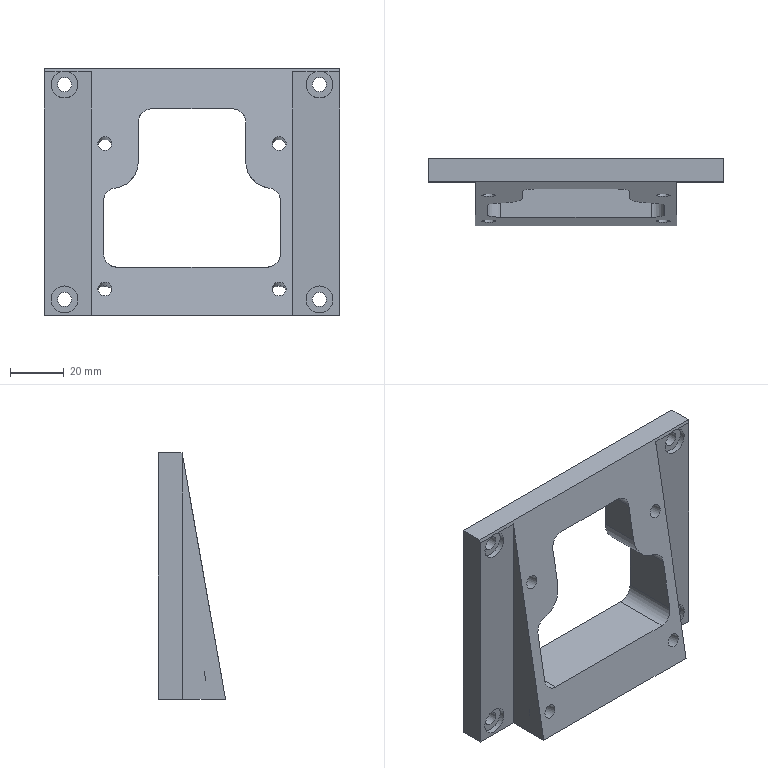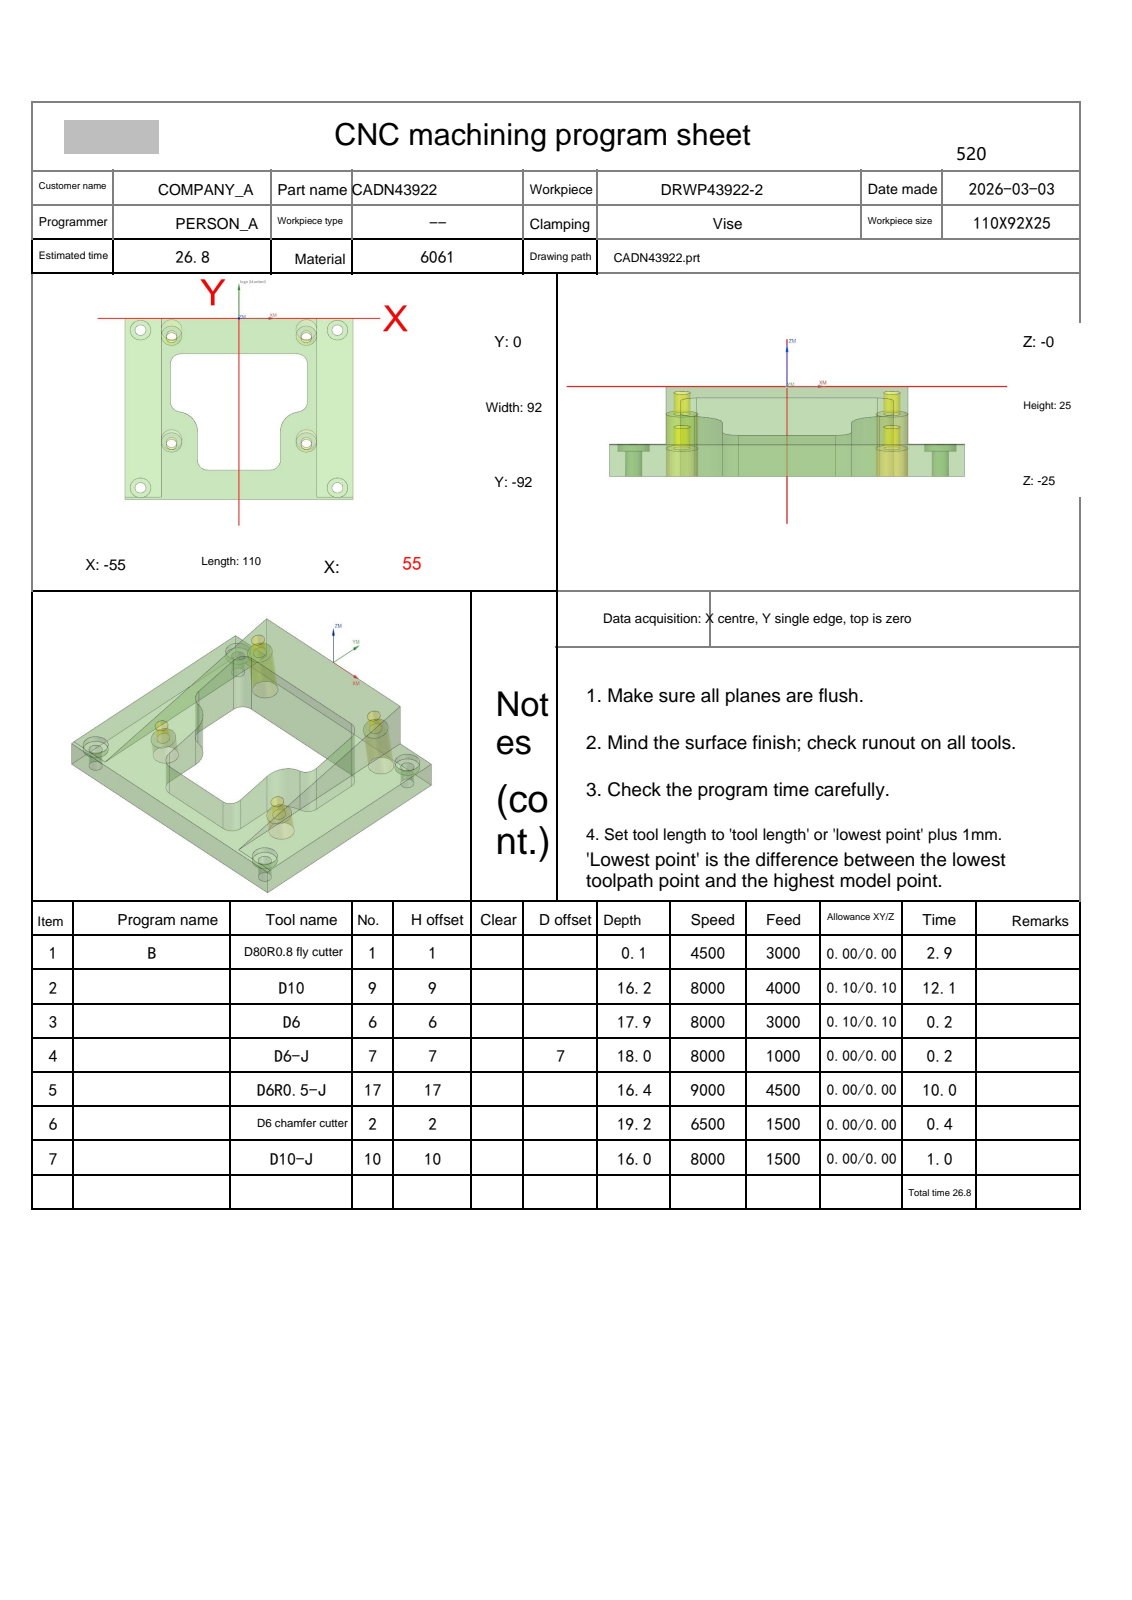NC program | NX | posted by the shop | part box 110 x 25 x 92 mm
Lines 5947 to 7507 of 14355:
N5 T17 M06
(D6R0.5-J  D=6. R=0.5 H=17 ce=0.00 di=0.00)
G00 G90 G54 X38.576 Y-2.64 M03 S9000
G43 H17 Z14.5
M08
Z1.2
G01 Z-.017 F4500.
X37.5 Y-2.642
X-37.5
X-38.576 Y-2.64
Y-2.691 Z-.026
Y-2.739 Z-.035
X-37.5 Y-2.741
X37.5
X38.576 Y-2.739
X38.577 Y-2.79 Z-.043
Y-2.837 Z-.052
X37.5 Y-2.839
X-37.5
X-38.577 Y-2.837
Y-2.888 Z-.061
Y-2.936 Z-.069
X-37.5 Y-2.938
X37.5
X38.577 Y-2.936
X38.578 Y-2.987 Z-.078
Y-3.034 Z-.087
X37.5 Y-3.036
X-37.5
X-38.578 Y-3.034
Y-3.085 Z-.096
X-38.579 Y-3.133 Z-.104
X-37.5 Y-3.135
X37.5
X38.579 Y-3.133
Y-3.184 Z-.113
Y-3.231 Z-.122
X37.5 Y-3.233
X-37.5
X-38.579 Y-3.231
Y-3.282 Z-.13
X-38.58 Y-3.33 Z-.139
X-37.5 Y-3.332
X37.5
X38.58 Y-3.33
Y-3.381 Z-.148
Y-3.428 Z-.156
X37.5 Y-3.43
X-37.5
X-38.58 Y-3.428
Y-3.479 Z-.165
X-38.581 Y-3.527 Z-.174
X-37.5 Y-3.529
X37.5
X38.581 Y-3.527
Y-3.578 Z-.182
Y-3.625 Z-.191
X37.5 Y-3.627
X-37.5
X-38.581 Y-3.625
Y-3.676 Z-.2
X-38.582 Y-3.723 Z-.208
X-37.5 Y-3.726
X37.5
X38.582 Y-3.723
Y-3.775 Z-.217
Y-3.822 Z-.226
X37.5 Y-3.824
X-37.5
X-38.582 Y-3.822
X-38.583 Y-3.873 Z-.234
Y-3.92 Z-.243
X-37.5 Y-3.922
X37.5
X38.583 Y-3.92
Y-3.972 Z-.252
Y-4.019 Z-.26
X37.5 Y-4.021
X-37.5
X-38.583 Y-4.019
X-38.584 Y-4.07 Z-.269
Y-4.117 Z-.278
X-37.5 Y-4.119
X37.5
X38.584 Y-4.117
Y-4.169 Z-.287
Y-4.216 Z-.295
X37.5 Y-4.218
X-37.5
X-38.584 Y-4.216
X-38.585 Y-4.267 Z-.304
Y-4.314 Z-.313
X-37.5 Y-4.316
X37.5
X38.585 Y-4.314
Y-4.366 Z-.321
Y-4.413 Z-.33
X37.5 Y-4.415
X-37.5
X-38.585 Y-4.413
X-38.586 Y-4.464 Z-.339
Y-4.511 Z-.347
X-37.5 Y-4.513
X37.5
X38.586 Y-4.511
Y-4.563 Z-.356
Y-4.61 Z-.365
X37.5 Y-4.612
X-37.5
X-38.586 Y-4.61
Y-4.661 Z-.373
X-38.587 Y-4.708 Z-.382
X-37.5 Y-4.71
X37.5
X38.587 Y-4.708
Y-4.76 Z-.391
Y-4.807 Z-.399
X37.5 Y-4.809
X-37.5
X-38.587 Y-4.807
Y-4.858 Z-.408
X-38.588 Y-4.905 Z-.417
X-37.5 Y-4.907
X37.5
X38.588 Y-4.905
Y-4.957 Z-.425
Y-5.004 Z-.434
X37.5 Y-5.006
X-37.5
X-38.588 Y-5.004
Y-5.055 Z-.443
Y-5.102 Z-.451
X-37.5 Y-5.104
X37.5
X38.588 Y-5.102
X38.589 Y-5.153 Z-.46
Y-5.201 Z-.469
X37.5 Y-5.203
X-37.5
X-38.589 Y-5.201
Y-5.252 Z-.478
Y-5.299 Z-.486
X-37.5 Y-5.301
X37.5
X38.589 Y-5.299
Y-5.35 Z-.495
Y-5.398 Z-.504
X37.5 Y-5.4
X-37.5
X-38.589 Y-5.398
X-38.59 Y-5.449 Z-.512
Y-5.496 Z-.521
X-37.5 Y-5.498
X37.5
X38.59 Y-5.496
Y-5.547 Z-.53
Y-5.595 Z-.538
X37.5 Y-5.597
X-37.5
X-38.59 Y-5.595
Y-5.646 Z-.547
X-38.591 Y-5.693 Z-.556
X-37.5 Y-5.695
X37.5
X38.591 Y-5.693
Y-5.744 Z-.564
Y-5.792 Z-.573
X37.5 Y-5.794
X-37.5
X-38.591 Y-5.792
Y-5.843 Z-.582
Y-5.89 Z-.59
X-37.5 Y-5.892
X37.5
X38.591 Y-5.89
X38.592 Y-5.941 Z-.599
Y-5.989 Z-.608
X37.5 Y-5.991
X-37.5
X-38.592 Y-5.989
Y-6.04 Z-.616
Y-6.087 Z-.625
X-37.5 Y-6.089
X37.5
X38.592 Y-6.087
Y-6.138 Z-.634
X38.593 Y-6.186 Z-.642
X37.5 Y-6.188
X-37.5
X-38.593 Y-6.186
Y-6.237 Z-.651
Y-6.284 Z-.66
X-37.5 Y-6.286
X37.5
X38.593 Y-6.284
Y-6.335 Z-.669
Y-6.383 Z-.677
X37.5 Y-6.384
X-37.5
X-38.593 Y-6.383
Y-6.434 Z-.686
X-38.594 Y-6.481 Z-.695
X-37.5 Y-6.483
X37.5
X38.594 Y-6.481
Y-6.532 Z-.703
Y-6.58 Z-.712
X37.5 Y-6.581
X-37.5
X-38.594 Y-6.58
Y-6.631 Z-.721
Y-6.678 Z-.729
X-37.5 Y-6.68
X37.5
X38.594 Y-6.678
Y-6.729 Z-.738
Y-6.777 Z-.747
X37.5 Y-6.778
X-37.5
X-38.594 Y-6.777
Y-6.828 Z-.755
Y-6.875 Z-.764
X-37.5 Y-6.877
X37.5
X38.594 Y-6.875
X38.595 Y-6.926 Z-.773
Y-6.974 Z-.781
X37.5 Y-6.975
X-37.5
X-38.595 Y-6.974
Y-7.025 Z-.79
Y-7.072 Z-.799
X-37.5 Y-7.074
X37.5
X38.595 Y-7.072
Y-7.123 Z-.807
Y-7.171 Z-.816
X37.5 Y-7.172
X-37.5
X-38.595 Y-7.171
Y-7.222 Z-.825
Y-7.269 Z-.834
X-37.5 Y-7.271
X37.5
X38.595 Y-7.269
Y-7.32 Z-.842
Y-7.368 Z-.851
X37.5 Y-7.369
X-37.5
X-38.595 Y-7.368
X-38.596 Y-7.419 Z-.86
Y-7.466 Z-.868
X-37.5 Y-7.468
X37.5
X38.596 Y-7.466
Y-7.517 Z-.877
Y-7.565 Z-.886
X37.5 Y-7.566
X-37.5
X-38.596 Y-7.565
Y-7.616 Z-.894
Y-7.663 Z-.903
X-37.5 Y-7.665
X37.5
X38.596 Y-7.663
Y-7.714 Z-.912
Y-7.762 Z-.92
X37.5 Y-7.763
X-37.5
X-38.596 Y-7.762
Y-7.812 Z-.929
Y-7.86 Z-.938
X-37.5 Y-7.862
X37.5
X38.596 Y-7.86
X38.597 Y-7.911 Z-.946
Y-7.958 Z-.955
X37.5 Y-7.96
X-37.5
X-38.597 Y-7.958
Y-8.009 Z-.964
Y-8.057 Z-.972
X-37.5 Y-8.059
X37.5
X38.597 Y-8.057
Y-8.108 Z-.981
Y-8.155 Z-.99
X37.5 Y-8.157
X-37.5
X-38.597 Y-8.155
Y-8.206 Z-.998
Y-8.254 Z-1.007
X-37.5 Y-8.256
X37.5
X38.597 Y-8.254
Y-8.305 Z-1.016
X38.598 Y-8.352 Z-1.025
X37.5 Y-8.354
X-37.5
X-38.597 Y-8.352
Y-8.403 Z-1.033
Y-8.451 Z-1.042
X-37.5 Y-8.453
X37.5
X38.598 Y-8.451
Y-8.502 Z-1.051
Y-8.549 Z-1.059
X37.5 Y-8.551
X-37.5
X-38.598 Y-8.549
Y-8.6 Z-1.068
Y-8.648 Z-1.077
X-37.5 Y-8.65
X37.5
X38.598 Y-8.648
Y-8.699 Z-1.085
Y-8.746 Z-1.094
X37.5 Y-8.748
X-37.5
X-38.598 Y-8.746
Y-8.797 Z-1.103
Y-8.845 Z-1.111
X-37.5 Y-8.847
X37.5
X38.598 Y-8.845
Y-8.896 Z-1.12
Y-8.943 Z-1.129
X37.5 Y-8.945
X-37.5
X-38.598 Y-8.943
Y-8.994 Z-1.137
Y-9.042 Z-1.146
X-37.5 Y-9.043
X37.5
X38.598 Y-9.042
Y-9.093 Z-1.155
Y-9.14 Z-1.163
X37.5 Y-9.142
X-37.5
X-38.598 Y-9.14
Y-9.191 Z-1.172
Y-9.239 Z-1.181
X-37.5 Y-9.24
X37.5
X38.598 Y-9.239
Y-9.29 Z-1.189
Y-9.337 Z-1.198
X37.5 Y-9.339
X-37.5
X-38.598 Y-9.337
Y-9.388 Z-1.207
Y-9.436 Z-1.216
X-37.5 Y-9.437
X37.5
X38.598 Y-9.436
Y-9.487 Z-1.224
Y-9.534 Z-1.233
X37.5 Y-9.536
X-37.5
X-38.599 Y-9.534
Y-9.585 Z-1.242
Y-9.633 Z-1.25
X-37.5 Y-9.634
X37.5
X38.599 Y-9.633
Y-9.684 Z-1.259
Y-9.731 Z-1.268
X37.5 Y-9.733
X-37.5
X-38.599 Y-9.731
Y-9.782 Z-1.276
Y-9.83 Z-1.285
X-37.5 Y-9.831
X37.5
X38.599 Y-9.83
Y-9.881 Z-1.294
Y-9.928 Z-1.302
X37.5 Y-9.93
X-37.5
X-38.599 Y-9.928
Y-9.979 Z-1.311
Y-10.027 Z-1.32
X-37.5 Y-10.028
X37.5
X38.599 Y-10.027
Y-10.078 Z-1.328
Y-10.125 Z-1.337
X37.5 Y-10.127
X-37.5
X-38.599 Y-10.125
Y-10.176 Z-1.346
Y-10.224 Z-1.354
X-37.5 Y-10.225
X37.5
X38.599 Y-10.224
Y-10.274 Z-1.363
Y-10.322 Z-1.372
X37.5 Y-10.324
X-37.5
X-38.599 Y-10.322
Y-10.373 Z-1.381
Y-10.421 Z-1.389
X-37.5 Y-10.422
X37.5
X38.599 Y-10.421
Y-10.471 Z-1.398
Y-10.519 Z-1.407
X37.5 Y-10.521
X-37.5
X-38.599 Y-10.519
Y-10.57 Z-1.415
Y-10.618 Z-1.424
X-37.5 Y-10.619
X37.5
X38.599 Y-10.618
Y-10.668 Z-1.433
Y-10.716 Z-1.441
X37.5 Y-10.718
X-37.5
X-38.599 Y-10.716
Y-10.767 Z-1.45
Y-10.814 Z-1.459
X-37.5 Y-10.816
X37.5
X38.599 Y-10.814
Y-10.865 Z-1.467
Y-10.913 Z-1.476
X37.5 Y-10.915
X-37.5
X-38.599 Y-10.913
Y-10.964 Z-1.485
Y-11.011 Z-1.493
X-37.5 Y-11.013
X37.5
X38.599 Y-11.011
Y-11.062 Z-1.502
Y-11.11 Z-1.511
X37.5 Y-11.112
X34.721
X32.994 Y-11.109
G03 X32.501 Y-11.091 I-.493 J-6.934
X32.006 Y-11.109 I0.0 J-6.951
G01 X30.279 Y-11.112
X-30.279
X-32.006 Y-11.109
G03 X-32.501 Y-11.091 I-.495 J-6.928
X-32.994 Y-11.109 I0.0 J-6.946
G01 X-34.721 Y-11.112
X-37.5
X-38.599 Y-11.11
Y-11.161 Z-1.519
Y-11.208 Z-1.528
X-37.5 Y-11.21
X-34.778
X-33.203 Y-11.209
G02 X-32.499 Y-11.159 I.704 J-4.954
X-31.789 Y-11.209 I0.0 J-5.004
G01 X-30.222 Y-11.21
X30.222
X31.789 Y-11.209
G02 X32.499 Y-11.159 I.71 J-4.956
X33.204 Y-11.209 I0.0 J-5.006
G01 X34.778 Y-11.21
X37.5
X38.599 Y-11.208
Y-11.259 Z-1.537
Y-11.307 Z-1.545
X37.5 Y-11.309
X34.825
X33.335 Y-11.303
G03 X32.499 Y-11.223 I-.836 J-4.329
X31.66 Y-11.303 I0.0 J-4.409
G01 X30.175 Y-11.309
X-30.175
X-31.66 Y-11.303
G03 X-32.499 Y-11.223 I-.839 J-4.328
X-33.335 Y-11.303 I0.0 J-4.409
G01 X-34.825 Y-11.309
X-37.5
X-38.599 Y-11.307
Y-11.358 Z-1.554
Y-11.405 Z-1.563
X-37.5 Y-11.407
X-34.871
X-33.467 Y-11.404
X-32.49 Y-11.253
X-31.532 Y-11.403
X-30.129 Y-11.407
X30.129
X31.532 Y-11.403
X32.49 Y-11.253
X33.467 Y-11.404
X34.871 Y-11.407
X37.5
X38.6 Y-11.405
Y-11.456 Z-1.572
Y-11.504 Z-1.58
X37.5 Y-11.506
X34.918
X33.565 Y-11.504
G02 X32.49 Y-11.308 I.169 J3.981
X31.43 Y-11.505 I-1.183 J3.427
G01 X30.082 Y-11.506
X-30.082
X-31.43 Y-11.505
G02 X-32.49 Y-11.308 I.122 J3.616
X-33.565 Y-11.504 I-1.244 J3.785
G01 X-34.918 Y-11.506
X-37.5
X-38.599 Y-11.504
Y-11.555 Z-1.589
Y-11.602 Z-1.598
X-37.5 Y-11.604
X-34.955
X-33.637 Y-11.6
G03 X-32.49 Y-11.363 I-.32 J4.442
X-31.36 Y-11.601 I1.353 J3.628
G01 X-30.045 Y-11.604
X30.045
X31.36 Y-11.601
G03 X32.49 Y-11.363 I-.223 J3.865
X33.637 Y-11.6 I1.465 J4.199
G01 X34.955 Y-11.604
X37.5
X38.6 Y-11.602
Y-11.653 Z-1.606
Y-11.701 Z-1.615
X37.5 Y-11.702
X34.982
X33.709 Y-11.698
X33.661 Y-11.699
G02 X32.597 Y-11.445 I0.0 J2.36
G01 X32.5 Y-11.418
X32.404 Y-11.445
G02 X31.335 Y-11.699 I-1.069 J2.123
G01 X31.29
X30.018 Y-11.702
X-30.018
X-31.29 Y-11.699
X-31.335
G02 X-32.404 Y-11.445 I0.0 J2.377
G01 X-32.501 Y-11.418
X-32.598 Y-11.445
G02 X-33.66 Y-11.699 I-1.063 J2.102
G01 X-33.709 Y-11.698
X-34.982 Y-11.702
X-37.5
X-38.6 Y-11.701
Y-11.752 Z-1.624
Y-11.799 Z-1.632
X-37.5 Y-11.801
X-35.009
X-33.778 Y-11.798
X-33.757
G03 X-32.5 Y-11.478 I0.0 J2.631
X-31.245 Y-11.798 I1.255 J2.303
G01 X-31.223
X-29.991 Y-11.801
X29.991
X31.223 Y-11.798
X31.24
G03 X32.502 Y-11.479 I0.0 J2.66
X33.756 Y-11.798 I1.254 J2.309
G01 X33.778
X35.009 Y-11.801
X37.5
X38.6 Y-11.799
Y-11.85 Z-1.641
Y-11.898 Z-1.65
X37.5 Y-11.899
X35.036
X33.817 Y-11.897
G02 X32.502 Y-11.555 I.026 J2.8
X31.186 Y-11.896 I-1.353 J2.51
G01 X29.964 Y-11.899
X-29.964
X-31.186 Y-11.896
G02 X-32.5 Y-11.554 I.032 J2.815
X-33.817 Y-11.897 I-1.343 J2.458
G01 X-35.036 Y-11.899
X-37.5
X-38.6 Y-11.898
Y-11.949 Z-1.658
Y-11.996 Z-1.667
X-37.5 Y-11.998
X-35.062
X-33.857 Y-11.997
G03 X-32.5 Y-11.629 I-.028 J2.793
X-31.149 Y-11.996 I1.382 J2.421
G01 X-29.939 Y-11.998
X29.939
X31.149 Y-11.996
G03 X32.502 Y-11.63 I-.025 J2.781
X33.857 Y-11.997 I1.376 J2.398
G01 X35.062 Y-11.998
X37.5
X38.6 Y-11.996
Y-12.047 Z-1.676
Y-12.095 Z-1.684
X37.5 Y-12.096
X35.075
X33.889
G02 X32.502 Y-11.706 I.168 J3.259
X31.112 Y-12.096 I-1.607 J3.056
G01 X29.925
X-29.925
X-31.112
G02 X-32.5 Y-11.705 I.18 J3.296
X-33.889 Y-12.096 I-1.56 J2.877
G01 X-35.075
X-37.5
X-38.6 Y-12.095
Y-12.146 Z-1.693
Y-12.193 Z-1.702
X-37.5 Y-12.195
X-35.088
X-33.907
G03 X-32.5 Y-11.781 I-.001 J2.601
X-31.093 Y-12.195 I1.409 J2.191
G01 X-29.912
X29.912
X31.093
G03 X32.502 Y-11.782 I-.008 J2.637
X33.907 Y-12.195 I1.405 J2.186
G01 X35.088
X37.5
X38.6 Y-12.193
Y-12.244 Z-1.71
Y-12.292 Z-1.719
X37.5 Y-12.293
X35.094
X33.92
G02 X32.502 Y-11.873 I.044 J2.754
X31.08 Y-12.293 I-1.477 J2.383
G01 X29.906
X-29.906
X-31.08
G02 X-32.5 Y-11.872 I.048 J2.766
X-33.92 Y-12.293 I-1.464 J2.333
G01 X-35.094
X-37.5
X-38.6 Y-12.292
Y-12.343 Z-1.728
Y-12.39 Z-1.736
X-37.5 Y-12.392
X-35.098
X-33.933 Y-12.391
G03 X-32.5 Y-11.965 I-.014 J2.67
X-31.067 Y-12.391 I1.447 J2.243
G01 X-29.902 Y-12.392
X29.902
X31.067 Y-12.391
G03 X32.502 Y-11.967 I-.02 J2.701
X33.933 Y-12.391 I1.458 J2.291
G01 X35.098 Y-12.392
X37.5
X38.6 Y-12.39
Y-12.441 Z-1.745
Y-12.489 Z-1.754
X37.5 Y-12.49
X35.098
X33.943
X33.904
G02 X32.579 Y-12.094 I0.0 J2.412
G01 X32.529 Y-12.063
X32.47
X32.42 Y-12.094
G02 X31.096 Y-12.49 I-1.324 J2.014
G01 X31.057
X29.902
X-29.902
X-31.057
X-31.095
G02 X-32.43 Y-12.087 I0.0 J2.411
G01 X-32.473 Y-12.059
X-32.526
X-32.569 Y-12.087
G02 X-33.903 Y-12.49 I-1.334 J2.009
G01 X-33.942
X-35.098
X-37.5
X-38.6 Y-12.489
Y-12.54 Z-1.763
Y-12.587 Z-1.771
X-37.5 Y-12.589
X-35.093
X-33.922 Y-12.588
X-33.914
G03 X-32.5 Y-12.156 I0.0 J2.531
X-31.084 Y-12.589 I1.416 J2.103
G01 X-31.076
X-29.907
X29.907
X31.076
X31.079
G03 X32.502 Y-12.157 I0.0 J2.565
X33.914 Y-12.588 I1.412 J2.098
G01 X33.923
X35.093 Y-12.589
X37.5
X38.6 Y-12.587
Y-12.638 Z-1.78
Y-12.686 Z-1.789
X37.5 Y-12.687
X35.086
X33.903
G02 X32.502 Y-12.272 I.003 J2.581
X31.094 Y-12.687 I-1.416 J2.203
G01 X29.914
X-29.914
X-31.094
G02 X-32.5 Y-12.27 I.002 J2.588
X-33.903 Y-12.687 I-1.406 J2.166
G01 X-35.086
X-37.5
X-38.6 Y-12.686
Y-12.737 Z-1.797
Y-12.784 Z-1.806
X-37.5 Y-12.786
X-35.073
X-33.883
X-33.881
G03 X-32.5 Y-12.384 I0.0 J2.579
X-31.121 Y-12.785 I1.379 J2.171
G01 X-31.114
X-29.927 Y-12.786
X29.927
X31.114 Y-12.785
X31.116
G03 X32.502 Y-12.386 I0.0 J2.602
X33.881 Y-12.786 I1.379 J2.177
G01 X33.883
X35.073
X37.5
X38.6 Y-12.784
Y-12.835 Z-1.815
Y-12.883 Z-1.823
X37.5 Y-12.884
X35.059
X33.85 Y-12.883
X33.841
G02 X32.502 Y-12.501 I0.0 J2.54
X31.152 Y-12.882 I-1.35 J2.205
G01 X29.941 Y-12.884
X-29.941
X-31.151 Y-12.882
X-31.165
G02 X-32.5 Y-12.5 I0.0 J2.525
X-33.85 Y-12.883 I-1.353 J2.201
G01 X-35.059 Y-12.884
X-37.5
X-38.6 Y-12.883
Y-12.933 Z-1.832
Y-12.981 Z-1.841
X-37.5 Y-12.983
X-35.032
X-33.806 Y-12.98
X-33.799
G03 X-32.5 Y-12.625 I0.0 J2.553
X-31.204 Y-12.979 I1.296 J2.19
G01 X-31.194
X-29.968 Y-12.983
X29.968
X31.194 Y-12.979
X31.199
G03 X32.502 Y-12.626 I0.0 J2.578
X33.798 Y-12.98 I1.296 J2.197
G01 X33.806
X35.032 Y-12.983
X37.5
X38.6 Y-12.981
Y-13.032 Z-1.849
Y-13.08 Z-1.858
X37.5 Y-13.081
X35.006
X33.762 Y-13.078
X33.739
G02 X32.502 Y-12.75 I0.0 J2.498
X31.257 Y-13.078 I-1.245 J2.202
G01 X31.238 Y-13.077
X29.994 Y-13.081
X-29.994
X-31.238 Y-13.077
X-31.262 Y-13.078
G02 X-32.5 Y-12.749 I0.0 J2.497
X-33.739 Y-13.078 I-1.239 J2.172
G01 X-33.762
X-35.006 Y-13.081
X-37.5
X-38.6 Y-13.08
Y-13.13 Z-1.867
Y-13.178 Z-1.875
X-37.5 Y-13.18
X-34.979
X-33.716 Y-13.177
X-33.707
G03 X-32.49 Y-12.883 I0.0 J2.668
X-31.316 Y-13.177 I1.174 J2.196
G01 X-31.284
X-30.021 Y-13.18
X30.021
X31.284 Y-13.177
X31.316
G03 X32.49 Y-12.883 I0.0 J2.49
G01 X33.527 Y-13.173
X33.716 Y-13.177
X34.979 Y-13.18
X37.5
X38.6 Y-13.178
Y-13.229 Z-1.884
Y-13.277 Z-1.893
X37.5 Y-13.278
X34.952
X33.637 Y-13.275
X33.527 Y-13.274
X32.49 Y-13.019
X31.453 Y-13.275
X31.361 Y-13.276
X30.048 Y-13.278
X-30.048
X-31.361 Y-13.276
X-31.453 Y-13.275
X-32.49 Y-13.019
X-33.527 Y-13.274
X-33.637 Y-13.275
X-34.952 Y-13.278
X-37.5
X-38.6 Y-13.277
Y-13.327 Z-1.901
Y-13.375 Z-1.91
X-37.5 Y-13.377
X-34.912
X-33.558 Y-13.376
X-32.49 Y-13.156
X-31.438 Y-13.376
X-30.088 Y-13.377
X30.088
X31.438 Y-13.376
X32.49 Y-13.156
X33.558 Y-13.376
X34.912 Y-13.377
X37.5
X38.6 Y-13.375
Y-13.426 Z-1.919
Y-13.473 Z-1.927
X37.5 Y-13.475
X34.865
X33.467 Y-13.472
G03 X32.499 Y-13.362 I-.968 J-4.208
X31.533 Y-13.472 I0.0 J-4.318
G01 X30.135 Y-13.475
X-30.135
X-31.533 Y-13.472
G03 X-32.499 Y-13.362 I-.966 J-4.208
X-33.467 Y-13.472 I0.0 J-4.318
G01 X-34.865 Y-13.475
X-37.5
X-38.6 Y-13.473
Y-13.524 Z-1.936
Y-13.572 Z-1.945
X-37.5 Y-13.574
X-34.819
X-33.338 Y-13.57
G02 X-32.5 Y-13.49 I.838 J-4.356
X-31.66 Y-13.57 I0.0 J-4.436
G01 X-30.181 Y-13.574
X30.181
X31.659 Y-13.57
G02 X32.5 Y-13.49 I.84 J-4.356
X33.338 Y-13.57 I0.0 J-4.436
G01 X34.819 Y-13.574
X37.5
X38.6 Y-13.572
Y-13.623 Z-1.954
Y-13.67 Z-1.962
X37.5 Y-13.672
X34.772
X33.188
G03 X32.498 Y-13.613 I-.69 J-4.006
X31.812 Y-13.671 I0.0 J-4.065
G01 X30.228 Y-13.672
X-30.228
X-31.812 Y-13.671
G03 X-32.498 Y-13.613 I-.686 J-4.002
X-33.188 Y-13.672 I0.0 J-4.061
G01 X-34.772
X-37.5
X-38.6 Y-13.67
Y-13.721 Z-1.971
Y-13.769 Z-1.98
X-37.5 Y-13.771
X-34.712
X-32.928 Y-13.765
X-32.069 Y-13.766
X-30.288 Y-13.771
X30.288
X32.069 Y-13.766
X32.928 Y-13.765
X34.712 Y-13.771
X37.5
X38.6 Y-13.769
Y-13.82 Z-1.988
Y-13.867 Z-1.997
X37.5 Y-13.869
X-37.5
X-38.6 Y-13.867
Y-13.918 Z-2.006
Y-13.966 Z-2.014
X-37.5 Y-13.968
X37.5
X38.6 Y-13.966
Y-14.017 Z-2.023
Y-14.064 Z-2.032
X37.5 Y-14.066
X-37.5
X-38.6 Y-14.064
Y-14.115 Z-2.04
Y-14.163 Z-2.049
X-37.5 Y-14.164
X37.5
X38.6 Y-14.163
Y-14.214 Z-2.058
Y-14.261 Z-2.066
X37.5 Y-14.263
X-37.5
X-38.6 Y-14.261
Y-14.312 Z-2.075
Y-14.36 Z-2.084
X-37.5 Y-14.361
X37.5
X38.6 Y-14.36
Y-14.411 Z-2.092
Y-14.458 Z-2.101
X37.5 Y-14.46
X-37.5
X-38.6 Y-14.458
Y-14.509 Z-2.11
Y-14.557 Z-2.119
X-37.5 Y-14.558
X37.5
X38.6 Y-14.557
Y-14.608 Z-2.127
Y-14.655 Z-2.136
X37.5 Y-14.657
X-37.5
X-38.6 Y-14.655
Y-14.706 Z-2.145
Y-14.754 Z-2.153
X-37.5 Y-14.755
X37.5
X38.6 Y-14.754
Y-14.805 Z-2.162
Y-14.852 Z-2.171
X37.5 Y-14.854
X-37.5
X-38.6 Y-14.852
Y-14.903 Z-2.179
Y-14.951 Z-2.188
X-37.5 Y-14.952
X37.5
X38.6 Y-14.951
Y-15.002 Z-2.197
Y-15.049 Z-2.205
X37.5 Y-15.051
X-37.5
X-38.6 Y-15.049
Y-15.1 Z-2.214
Y-15.148 Z-2.223
X-37.5 Y-15.149
X37.5
X38.6 Y-15.148
Y-15.199 Z-2.231
Y-15.247 Z-2.24
X37.5 Y-15.248
X-37.5
X-38.6 Y-15.247
Y-15.297 Z-2.249
Y-15.345 Z-2.257
X-37.5 Y-15.346
X37.5
X38.6 Y-15.345
Y-15.395 Z-2.266
Y-15.443 Z-2.275
X37.5 Y-15.445
X-37.5
X-38.6 Y-15.443
Y-15.494 Z-2.283
Y-15.542 Z-2.292
X-37.5 Y-15.543
X37.5
X38.6 Y-15.542
Y-15.592 Z-2.301
Y-15.64 Z-2.31
X37.5 Y-15.642
X-37.5
X-38.6 Y-15.64
Y-15.691 Z-2.318
Y-15.739 Z-2.327
X-37.5 Y-15.74
X37.5
X38.6 Y-15.739
Y-15.789 Z-2.336
Y-15.837 Z-2.344
X37.5 Y-15.839
X-37.5
X-38.6 Y-15.837
Y-15.888 Z-2.353
Y-15.936 Z-2.362
X-37.5 Y-15.937
X37.5
X38.6 Y-15.936
Y-15.986 Z-2.37
Y-16.034 Z-2.379
X37.5 Y-16.036
X-37.5
X-38.6 Y-16.034
Y-16.085 Z-2.388
Y-16.132 Z-2.396
X-37.5 Y-16.134
X37.5
X38.6 Y-16.132
Y-16.183 Z-2.405
Y-16.231 Z-2.414
X37.5 Y-16.233
X-37.5
X-38.6 Y-16.231
Y-16.282 Z-2.422
Y-16.329 Z-2.431
X-37.5 Y-16.331
X37.5
X38.6 Y-16.329
Y-16.38 Z-2.44
Y-16.428 Z-2.448
X37.5 Y-16.43
X-37.5
X-38.6 Y-16.428
Y-16.479 Z-2.457
Y-16.526 Z-2.466
X-37.5 Y-16.528
X37.5
X38.6 Y-16.526
Y-16.577 Z-2.474
Y-16.625 Z-2.483
X37.5 Y-16.627
X-37.5
X-38.6 Y-16.625
Y-16.676 Z-2.492
Y-16.723 Z-2.501
X-37.5 Y-16.725
X37.5
X38.6 Y-16.723
Y-16.774 Z-2.509
Y-16.822 Z-2.518
X37.5 Y-16.823
X-37.5
X-38.6 Y-16.822
Y-16.873 Z-2.527
Y-16.92 Z-2.535
X-37.5 Y-16.922
X37.5
X38.6 Y-16.92
Y-16.971 Z-2.544
Y-17.019 Z-2.553
X37.5 Y-17.02
X-37.5
X-38.6 Y-17.019
Y-17.07 Z-2.561
Y-17.117 Z-2.57
X-37.5 Y-17.119
X37.5
X38.6 Y-17.117
Y-17.168 Z-2.579
Y-17.216 Z-2.587
X37.5 Y-17.217
X-37.5
X-38.6 Y-17.216
Y-17.267 Z-2.596
Y-17.314 Z-2.605
X-37.5 Y-17.316
X37.5
X38.6 Y-17.314
Y-17.365 Z-2.613
Y-17.413 Z-2.622
X37.5 Y-17.414
X-37.5
X-38.6 Y-17.413
Y-17.464 Z-2.631
Y-17.511 Z-2.639
X-37.5 Y-17.513
X37.5
X38.6 Y-17.511
Y-17.562 Z-2.648
Y-17.61 Z-2.657
X37.5 Y-17.611
X-37.5
X-38.6 Y-17.61
Y-17.661 Z-2.666
Y-17.708 Z-2.674
X-37.5 Y-17.71
X37.5
X38.6 Y-17.708
Y-17.759 Z-2.683
Y-17.807 Z-2.692
X37.5 Y-17.808
X-37.5
X-38.6 Y-17.807
Y-17.858 Z-2.7
Y-17.905 Z-2.709
X-37.5 Y-17.907
X37.5
X38.6 Y-17.905
Y-17.956 Z-2.718
Y-18.004 Z-2.726
X37.5 Y-18.005
X-37.5
X-38.6 Y-18.004
Y-18.054 Z-2.735
Y-18.102 Z-2.744
X-37.5 Y-18.104
X37.5
X38.6 Y-18.102
Y-18.153 Z-2.752
Y-18.201 Z-2.761
X37.5 Y-18.202
X-37.5
X-38.6 Y-18.201
Y-18.251 Z-2.77
Y-18.299 Z-2.778
X-37.5 Y-18.301
X37.5
X38.6 Y-18.299
Y-18.35 Z-2.787
Y-18.398 Z-2.796
X37.5 Y-18.399
X-37.5
X-38.6 Y-18.398
Y-18.448 Z-2.804
Y-18.496 Z-2.813
X-37.5 Y-18.498
X37.5
X38.6 Y-18.496
Y-18.547 Z-2.822
Y-18.594 Z-2.83
X37.5 Y-18.596
X-37.5
X-38.6 Y-18.594
Y-18.645 Z-2.839
Y-18.693 Z-2.848
X-37.5 Y-18.695
X37.5
X38.6 Y-18.693
Y-18.744 Z-2.857
Y-18.791 Z-2.865
X37.5 Y-18.793
X-37.5
X-38.6 Y-18.791
Y-18.842 Z-2.874
Y-18.89 Z-2.883
X-37.5 Y-18.892
X37.5
X38.6 Y-18.89
Y-18.941 Z-2.891
Y-18.988 Z-2.9
X37.5 Y-18.99
X-37.5
X-38.6 Y-18.988
Y-19.039 Z-2.909
Y-19.087 Z-2.917
X-37.5 Y-19.089
X37.5
X38.6 Y-19.087
Y-19.138 Z-2.926
Y-19.185 Z-2.935
X37.5 Y-19.187
X-37.5
X-38.6 Y-19.185
Y-19.236 Z-2.943
Y-19.284 Z-2.952
X-37.5 Y-19.285
X37.5
X38.6 Y-19.284
Y-19.335 Z-2.961
Y-19.382 Z-2.969
X37.5 Y-19.384
X-37.5
X-38.6 Y-19.382
Y-19.433 Z-2.978
Y-19.481 Z-2.987
X-37.5 Y-19.482
X37.5
X38.6 Y-19.481
Y-19.532 Z-2.995
Y-19.579 Z-3.004
X37.5 Y-19.581
X-37.5
X-38.6 Y-19.579
Y-19.63 Z-3.013
Y-19.678 Z-3.021
X-37.5 Y-19.679
X37.5
X38.6 Y-19.678
Y-19.729 Z-3.03
Y-19.776 Z-3.039
X37.5 Y-19.778
X-37.5
X-38.6 Y-19.776
Y-19.827 Z-3.048
Y-19.875 Z-3.056
X-37.5 Y-19.876
X37.5
X38.6 Y-19.875
Y-19.926 Z-3.065
Y-19.973 Z-3.074
X37.5 Y-19.975
X-37.5
X-38.6 Y-19.973
Y-20.024 Z-3.082
Y-20.072 Z-3.091
X-37.5 Y-20.073
X37.5
X38.6 Y-20.072
Y-20.123 Z-3.1
Y-20.17 Z-3.108
X37.5 Y-20.172
X-37.5
X-38.6 Y-20.17
Y-20.221 Z-3.117
Y-20.269 Z-3.126
X-37.5 Y-20.27
X37.5
X38.6 Y-20.269
Y-20.32 Z-3.134
Y-20.367 Z-3.143
X37.5 Y-20.369
X-37.5
X-38.6 Y-20.367
Y-20.418 Z-3.152
Y-20.466 Z-3.16
X-37.5 Y-20.467
X37.5
X38.6 Y-20.466
Y-20.517 Z-3.169
Y-20.564 Z-3.178
X37.5 Y-20.566
X-37.5
X-38.6 Y-20.564
Y-20.615 Z-3.186
Y-20.663 Z-3.195
X-37.5 Y-20.664
X37.5
X38.6 Y-20.663
Y-20.713 Z-3.204
Y-20.761 Z-3.212
X37.5 Y-20.763
X-37.5
X-38.6 Y-20.761
Y-20.812 Z-3.221
Y-20.86 Z-3.23
X-37.5 Y-20.861
X37.5
X38.6 Y-20.86
Y-20.91 Z-3.239
Y-20.958 Z-3.247
X37.5 Y-20.96
X-37.5
X-38.6 Y-20.958
Y-21.009 Z-3.256
Y-21.057 Z-3.265
X-37.5 Y-21.058
X37.5
X38.6 Y-21.057
Y-21.107 Z-3.273
Y-21.155 Z-3.282
X37.5 Y-21.157
X-37.5
X-38.6 Y-21.155
Y-21.206 Z-3.291
Y-21.253 Z-3.299
X-37.5 Y-21.255
X37.5
X38.6 Y-21.253
Y-21.304 Z-3.308
Y-21.352 Z-3.317
X37.5 Y-21.354
X-37.5
X-38.6 Y-21.352
Y-21.403 Z-3.325
Y-21.45 Z-3.334
X-37.5 Y-21.452
X37.5
X38.6 Y-21.45
Y-21.501 Z-3.343
Y-21.549 Z-3.351
X37.5 Y-21.551
X-37.5
X-38.6 Y-21.549
Y-21.6 Z-3.36
Y-21.647 Z-3.369
X-37.5 Y-21.649
X37.5
X38.6 Y-21.647
Y-21.698 Z-3.377
Y-21.746 Z-3.386
X37.5 Y-21.748
X31.199
X28.527 Y-21.744
X28.691 Y-21.78 Z-3.392
X28.855 Y-21.813 Z-3.398
X29.019 Y-21.845 Z-3.404
X31.317 Y-21.846
X37.5
X38.6 Y-21.844
Y-21.895 Z-3.412
Y-21.943 Z-3.421
X37.5 Y-21.944
X31.422
X29.323 Y-21.941
X29.441 Y-21.994 Z-3.43
X29.559 Y-22.036 Z-3.438
X29.725 Y-22.043
X37.5
X38.6 Y-22.041
Y-22.092 Z-3.447
Y-22.14 Z-3.456
X37.5 Y-22.141
X31.62
X29.774
X29.86 Y-22.191 Z-3.464
X29.946 Y-22.233 Z-3.473
X30.07 Y-22.24
X37.5
X38.6 Y-22.238
Y-22.289 Z-3.482
Y-22.337 Z-3.49
X37.5 Y-22.338
X31.799
X30.106 Y-22.337
X30.248 Y-22.432 Z-3.508
X31.881 Y-22.437
X37.5
X38.6 Y-22.435
Y-22.486 Z-3.516
Y-22.534 Z-3.525
X37.5 Y-22.535
X31.96
X30.384 Y-22.534
X30.497 Y-22.63 Z-3.542
X32.032 Y-22.634
X37.5
X38.6 Y-22.632
Y-22.683 Z-3.551
Y-22.731 Z-3.56
X37.5 Y-22.732
X32.104
X30.607 Y-22.727
X30.716 Y-22.828 Z-3.577
X32.169 Y-22.831
X37.5
X38.6 Y-22.829
Y-22.88 Z-3.586
Y-22.928 Z-3.595
X37.5 Y-22.929
X32.233
X30.809 Y-22.927
X30.895 Y-23.023 Z-3.612
X32.294 Y-23.028
X37.5
X38.6 Y-23.026
Y-23.077 Z-3.621
Y-23.125 Z-3.629
X37.5 Y-23.126
X32.35
X30.981 Y-23.122
X31.063 Y-23.222 Z-3.647
X32.406 Y-23.225
X37.5
X38.6 Y-23.223
Y-23.274 Z-3.655
Y-23.322 Z-3.664
X37.5 Y-23.323
X32.456
X31.133 Y-23.322
X31.2 Y-23.419 Z-3.681
X32.504 Y-23.422
X37.5
X38.6 Y-23.42
Y-23.471 Z-3.69
Y-23.519 Z-3.699
X37.5 Y-23.52
X32.552
X31.267 Y-23.517
X31.324 Y-23.615 Z-3.716
X32.594 Y-23.619
X37.5
X38.6 Y-23.617
Y-23.668 Z-3.725
Y-23.716 Z-3.733
X37.5 Y-23.717
X32.635
X31.379 Y-23.714
X31.433 Y-23.814 Z-3.751
X32.675 Y-23.816
X37.5
X38.6 Y-23.814
Y-23.865 Z-3.759
Y-23.912 Z-3.768
X37.5 Y-23.914
X32.71
X31.482
X31.525 Y-24.011 Z-3.786
X32.744 Y-24.013
X37.5
X38.6 Y-24.011
Y-24.062 Z-3.794
Y-24.109 Z-3.803
X37.5 Y-24.111
X32.777
X31.567 Y-24.109
X31.61 Y-24.207 Z-3.82
X32.804 Y-24.21
X37.5
X38.6 Y-24.208
Y-24.259 Z-3.829
Y-24.306 Z-3.838
X37.5 Y-24.308
X32.832
X31.643 Y-24.305
X31.674 Y-24.403 Z-3.855
X32.858 Y-24.406
X37.5
X38.6 Y-24.405
Y-24.456 Z-3.864
Y-24.503 Z-3.872
X37.5 Y-24.505
X32.879
X31.706 Y-24.502
X31.734 Y-24.601 Z-3.89
X32.9 Y-24.603
X37.5
X38.6 Y-24.602
Y-24.653 Z-3.898
Y-24.7 Z-3.907
X37.5 Y-24.702
X32.921
X31.757 Y-24.7
X31.769 Y-24.751 Z-3.916
X31.78 Y-24.799 Z-3.924
X32.936 Y-24.8
X37.5
X38.6 Y-24.799
Y-24.85 Z-3.933
Y-24.897 Z-3.942
X37.5 Y-24.899
X32.951
X31.801
X31.808 Y-24.948 Z-3.951
X31.815 Y-24.997 Z-3.959
X32.965
X37.5
X38.6 Y-24.996
Y-25.047 Z-3.968
Y-25.094 Z-3.977
X37.5 Y-25.096
X32.974
X31.827
X31.834 Y-25.145 Z-3.985
X31.84 Y-25.194 Z-3.994
X32.983
X37.5
X38.6 Y-25.193
Y-25.244 Z-4.003
Y-25.291 Z-4.011
X37.5 Y-25.293
X32.991
X31.85 Y-25.292
X31.853 Y-25.342 Z-4.02
X31.856 Y-25.391 Z-4.029
X32.994
X37.5
X38.6 Y-25.39
Y-25.441 Z-4.037
Y-25.488 Z-4.046
X37.5 Y-25.49
X32.997
X31.861 Y-25.489
X31.863 Y-25.539 Z-4.055
X31.866 Y-25.588 Z-4.063
X33.
X37.5
X38.6 Y-25.587
Y-25.638 Z-4.072
Y-25.685 Z-4.081
X37.5 Y-25.687
X33.
X31.868 Y-25.686
Y-25.736 Z-4.089
X31.869 Y-25.784 Z-4.098
X33. Y-25.785
X37.5
X38.6 Y-25.784
Y-25.834 Z-4.107
Y-25.882 Z-4.115
X37.5 Y-25.884
X33.
X31.869 Y-25.883
X31.87 Y-25.933 Z-4.124
Y-25.981 Z-4.133
X33. Y-25.982
X37.5
X38.6 Y-25.981
Y-26.031 Z-4.142
Y-26.079 Z-4.15
X37.5 Y-26.081
X33.
X31.871 Y-26.08
X31.872 Y-26.13 Z-4.159
Y-26.178 Z-4.168
X33. Y-26.179
X37.5
X38.6 Y-26.178
Y-26.228 Z-4.176
Y-26.276 Z-4.185
X37.5 Y-26.278
X33.
X31.873 Y-26.277
X31.874 Y-26.327 Z-4.194
Y-26.375 Z-4.202
X33. Y-26.376
X37.5
X38.6 Y-26.374
Y-26.425 Z-4.211
Y-26.473 Z-4.22
X37.5 Y-26.475
X33.
X31.875 Y-26.474
Y-26.524 Z-4.228
X31.876 Y-26.572 Z-4.237
X33. Y-26.573
X37.5
X38.6 Y-26.571
Y-26.622 Z-4.246
Y-26.67 Z-4.254
X37.5 Y-26.672
X33.
X31.877 Y-26.671
Y-26.721 Z-4.263
X31.878 Y-26.769 Z-4.272
X33. Y-26.77
X37.5
X38.6 Y-26.768
Y-26.819 Z-4.28
Y-26.867 Z-4.289
X37.5 Y-26.869
X33.
X31.878 Y-26.868
X31.879 Y-26.918 Z-4.298
Y-26.966 Z-4.306
X33. Y-26.967
X37.5
X38.6 Y-26.965
Y-27.016 Z-4.315